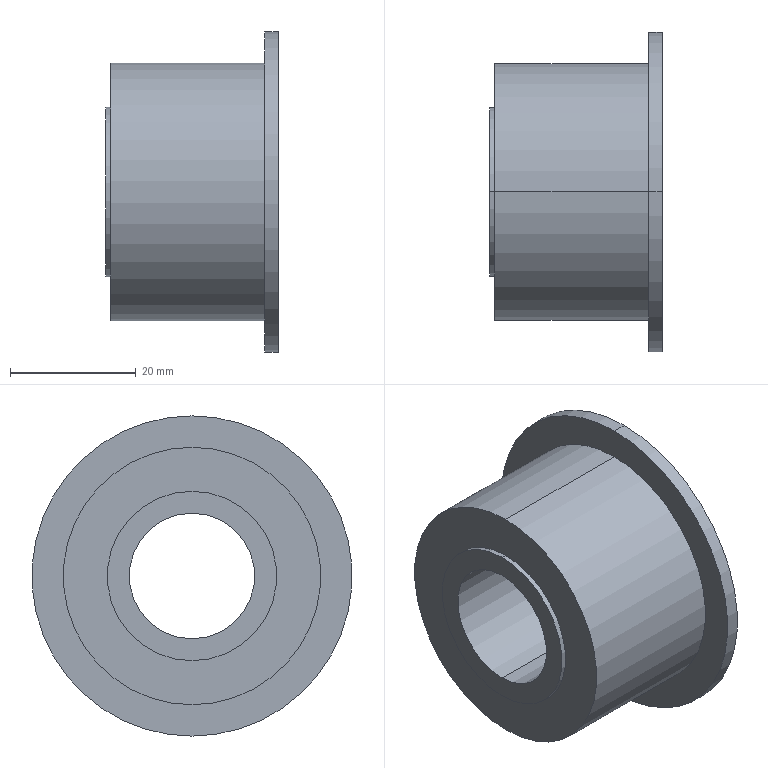Part | SolidWorks | features Revolution 1 | 1 solid | 18 faces | box 27.5 x 51 x 51 mm | volume 16998 mm3 | cylinder 12 | plane 6 | commonest cylinder face diameters 27 x4 20 x2 37 x2 41 x2 51 x2
STEP:
#1=CARTESIAN_POINT('',(27.5,0.,-18.5));
#2=VERTEX_POINT('',#1);
#3=CARTESIAN_POINT('',(27.5,0.,18.5));
#4=VERTEX_POINT('',#3);
#5=CARTESIAN_POINT('',(27.5,0.,0.));
#6=DIRECTION('',(-1.,0.,0.));
#7=DIRECTION('',(0.,0.,1.));
#8=AXIS2_PLACEMENT_3D('',#5,#6,#7);
#9=CIRCLE('',#8,18.5);
#10=EDGE_CURVE('',#2,#4,#9,.T.);
#11=ORIENTED_EDGE('',*,*,#10,.F.);
#12=CARTESIAN_POINT('',(4.3,0.,-18.5));
#13=VERTEX_POINT('',#12);
#14=CARTESIAN_POINT('',(0.,0.,-18.5));
#15=DIRECTION('',(-1.,0.,0.));
#16=VECTOR('',#15,1000.);
#17=LINE('',#14,#16);
#18=EDGE_CURVE('',#2,#13,#17,.T.);
#19=ORIENTED_EDGE('',*,*,#18,.T.);
#20=CARTESIAN_POINT('',(4.3,0.,18.5));
#21=VERTEX_POINT('',#20);
#22=CARTESIAN_POINT('',(4.3,0.,0.));
#23=DIRECTION('',(-1.,0.,0.));
#24=DIRECTION('',(0.,0.,1.));
#25=AXIS2_PLACEMENT_3D('',#22,#23,#24);
#26=CIRCLE('',#25,18.5);
#27=EDGE_CURVE('',#13,#21,#26,.T.);
#28=ORIENTED_EDGE('',*,*,#27,.T.);
#29=CARTESIAN_POINT('',(0.,0.,18.5));
#30=DIRECTION('',(-1.,0.,0.));
#31=VECTOR('',#30,1000.);
#32=LINE('',#29,#31);
#33=EDGE_CURVE('',#4,#21,#32,.T.);
#34=ORIENTED_EDGE('',*,*,#33,.F.);
#35=EDGE_LOOP('',(#11,#19,#28,#34));
#36=FACE_OUTER_BOUND('',#35,.T.);
#37=CARTESIAN_POINT('',(0.,0.,0.));
#38=DIRECTION('',(-1.,0.,0.));
#39=DIRECTION('',(0.,0.,1.));
#40=AXIS2_PLACEMENT_3D('',#37,#38,#39);
#41=CYLINDRICAL_SURFACE('',#40,18.5);
#42=ADVANCED_FACE('',(#36),#41,.F.);
#43=CARTESIAN_POINT('',(27.5,0.,13.5));
#44=VERTEX_POINT('',#43);
#45=CARTESIAN_POINT('',(27.5,0.,-13.5));
#46=VERTEX_POINT('',#45);
#47=CARTESIAN_POINT('',(27.5,0.,0.));
#48=DIRECTION('',(-1.,0.,0.));
#49=DIRECTION('',(0.,0.,1.));
#50=AXIS2_PLACEMENT_3D('',#47,#48,#49);
#51=CIRCLE('',#50,13.5);
#52=EDGE_CURVE('',#44,#46,#51,.T.);
#53=ORIENTED_EDGE('',*,*,#52,.T.);
#54=CARTESIAN_POINT('',(4.3,0.,-13.5));
#55=VERTEX_POINT('',#54);
#56=CARTESIAN_POINT('',(0.,0.,-13.5));
#57=DIRECTION('',(-1.,0.,0.));
#58=VECTOR('',#57,1000.);
#59=LINE('',#56,#58);
#60=EDGE_CURVE('',#46,#55,#59,.T.);
#61=ORIENTED_EDGE('',*,*,#60,.T.);
#62=CARTESIAN_POINT('',(4.3,0.,13.5));
#63=VERTEX_POINT('',#62);
#64=CARTESIAN_POINT('',(4.3,0.,0.));
#65=DIRECTION('',(-1.,0.,0.));
#66=DIRECTION('',(0.,0.,1.));
#67=AXIS2_PLACEMENT_3D('',#64,#65,#66);
#68=CIRCLE('',#67,13.5);
#69=EDGE_CURVE('',#63,#55,#68,.T.);
#70=ORIENTED_EDGE('',*,*,#69,.F.);
#71=CARTESIAN_POINT('',(0.,0.,13.5));
#72=DIRECTION('',(-1.,0.,0.));
#73=VECTOR('',#72,1000.);
#74=LINE('',#71,#73);
#75=EDGE_CURVE('',#44,#63,#74,.T.);
#76=ORIENTED_EDGE('',*,*,#75,.F.);
#77=EDGE_LOOP('',(#53,#61,#70,#76));
#78=FACE_OUTER_BOUND('',#77,.T.);
#79=CARTESIAN_POINT('',(0.,0.,0.));
#80=DIRECTION('',(-1.,0.,0.));
#81=DIRECTION('',(0.,0.,1.));
#82=AXIS2_PLACEMENT_3D('',#79,#80,#81);
#83=CYLINDRICAL_SURFACE('',#82,13.5);
#84=ADVANCED_FACE('',(#78),#83,.T.);
#85=CARTESIAN_POINT('',(27.5,0.,-10.));
#86=VERTEX_POINT('',#85);
#87=CARTESIAN_POINT('',(27.5,0.,10.));
#88=VERTEX_POINT('',#87);
#89=CARTESIAN_POINT('',(27.5,0.,0.));
#90=DIRECTION('',(-1.,0.,0.));
#91=DIRECTION('',(0.,0.,1.));
#92=AXIS2_PLACEMENT_3D('',#89,#90,#91);
#93=CIRCLE('',#92,10.);
#94=EDGE_CURVE('',#86,#88,#93,.T.);
#95=ORIENTED_EDGE('',*,*,#94,.F.);
#96=CARTESIAN_POINT('',(0.,0.,-10.));
#97=VERTEX_POINT('',#96);
#98=CARTESIAN_POINT('',(0.,0.,-10.));
#99=DIRECTION('',(-1.,0.,0.));
#100=VECTOR('',#99,1000.);
#101=LINE('',#98,#100);
#102=EDGE_CURVE('',#86,#97,#101,.T.);
#103=ORIENTED_EDGE('',*,*,#102,.T.);
#104=CARTESIAN_POINT('',(0.,0.,10.));
#105=VERTEX_POINT('',#104);
#106=CARTESIAN_POINT('',(0.,0.,0.));
#107=DIRECTION('',(-1.,0.,0.));
#108=DIRECTION('',(0.,0.,1.));
#109=AXIS2_PLACEMENT_3D('',#106,#107,#108);
#110=CIRCLE('',#109,10.);
#111=EDGE_CURVE('',#97,#105,#110,.T.);
#112=ORIENTED_EDGE('',*,*,#111,.T.);
#113=CARTESIAN_POINT('',(0.,0.,10.));
#114=DIRECTION('',(-1.,0.,0.));
#115=VECTOR('',#114,1000.);
#116=LINE('',#113,#115);
#117=EDGE_CURVE('',#88,#105,#116,.T.);
#118=ORIENTED_EDGE('',*,*,#117,.F.);
#119=EDGE_LOOP('',(#95,#103,#112,#118));
#120=FACE_OUTER_BOUND('',#119,.T.);
#121=CARTESIAN_POINT('',(0.,0.,0.));
#122=DIRECTION('',(-1.,0.,0.));
#123=DIRECTION('',(0.,0.,1.));
#124=AXIS2_PLACEMENT_3D('',#121,#122,#123);
#125=CYLINDRICAL_SURFACE('',#124,10.);
#126=ADVANCED_FACE('',(#120),#125,.F.);
#127=CARTESIAN_POINT('',(0.8,0.,13.5));
#128=VERTEX_POINT('',#127);
#129=CARTESIAN_POINT('',(0.8,0.,-13.5));
#130=VERTEX_POINT('',#129);
#131=CARTESIAN_POINT('',(0.8,0.,0.));
#132=DIRECTION('',(-1.,0.,0.));
#133=DIRECTION('',(0.,0.,1.));
#134=AXIS2_PLACEMENT_3D('',#131,#132,#133);
#135=CIRCLE('',#134,13.5);
#136=EDGE_CURVE('',#128,#130,#135,.T.);
#137=ORIENTED_EDGE('',*,*,#136,.T.);
#138=CARTESIAN_POINT('',(0.,0.,-13.5));
#139=VERTEX_POINT('',#138);
#140=CARTESIAN_POINT('',(0.,0.,-13.5));
#141=DIRECTION('',(-1.,0.,0.));
#142=VECTOR('',#141,1000.);
#143=LINE('',#140,#142);
#144=EDGE_CURVE('',#130,#139,#143,.T.);
#145=ORIENTED_EDGE('',*,*,#144,.T.);
#146=CARTESIAN_POINT('',(0.,0.,13.5));
#147=VERTEX_POINT('',#146);
#148=CARTESIAN_POINT('',(0.,0.,0.));
#149=DIRECTION('',(-1.,0.,0.));
#150=DIRECTION('',(0.,0.,1.));
#151=AXIS2_PLACEMENT_3D('',#148,#149,#150);
#152=CIRCLE('',#151,13.5);
#153=EDGE_CURVE('',#147,#139,#152,.T.);
#154=ORIENTED_EDGE('',*,*,#153,.F.);
#155=CARTESIAN_POINT('',(0.,0.,13.5));
#156=DIRECTION('',(-1.,0.,0.));
#157=VECTOR('',#156,1000.);
#158=LINE('',#155,#157);
#159=EDGE_CURVE('',#128,#147,#158,.T.);
#160=ORIENTED_EDGE('',*,*,#159,.F.);
#161=EDGE_LOOP('',(#137,#145,#154,#160));
#162=FACE_OUTER_BOUND('',#161,.T.);
#163=CARTESIAN_POINT('',(0.,0.,0.));
#164=DIRECTION('',(-1.,0.,0.));
#165=DIRECTION('',(0.,0.,1.));
#166=AXIS2_PLACEMENT_3D('',#163,#164,#165);
#167=CYLINDRICAL_SURFACE('',#166,13.5);
#168=ADVANCED_FACE('',(#162),#167,.T.);
#169=CARTESIAN_POINT('',(25.3,0.,20.5));
#170=VERTEX_POINT('',#169);
#171=CARTESIAN_POINT('',(25.3,0.,-20.5));
#172=VERTEX_POINT('',#171);
#173=CARTESIAN_POINT('',(25.3,0.,0.));
#174=DIRECTION('',(-1.,0.,0.));
#175=DIRECTION('',(0.,0.,1.));
#176=AXIS2_PLACEMENT_3D('',#173,#174,#175);
#177=CIRCLE('',#176,20.5);
#178=EDGE_CURVE('',#170,#172,#177,.T.);
#179=ORIENTED_EDGE('',*,*,#178,.T.);
#180=CARTESIAN_POINT('',(0.8,0.,-20.5));
#181=VERTEX_POINT('',#180);
#182=CARTESIAN_POINT('',(0.,0.,-20.5));
#183=DIRECTION('',(-1.,0.,0.));
#184=VECTOR('',#183,1000.);
#185=LINE('',#182,#184);
#186=EDGE_CURVE('',#172,#181,#185,.T.);
#187=ORIENTED_EDGE('',*,*,#186,.T.);
#188=CARTESIAN_POINT('',(0.8,0.,20.5));
#189=VERTEX_POINT('',#188);
#190=CARTESIAN_POINT('',(0.8,0.,0.));
#191=DIRECTION('',(-1.,0.,0.));
#192=DIRECTION('',(0.,0.,1.));
#193=AXIS2_PLACEMENT_3D('',#190,#191,#192);
#194=CIRCLE('',#193,20.5);
#195=EDGE_CURVE('',#189,#181,#194,.T.);
#196=ORIENTED_EDGE('',*,*,#195,.F.);
#197=CARTESIAN_POINT('',(0.,0.,20.5));
#198=DIRECTION('',(-1.,0.,0.));
#199=VECTOR('',#198,1000.);
#200=LINE('',#197,#199);
#201=EDGE_CURVE('',#170,#189,#200,.T.);
#202=ORIENTED_EDGE('',*,*,#201,.F.);
#203=EDGE_LOOP('',(#179,#187,#196,#202));
#204=FACE_OUTER_BOUND('',#203,.T.);
#205=CARTESIAN_POINT('',(0.,0.,0.));
#206=DIRECTION('',(-1.,0.,0.));
#207=DIRECTION('',(0.,0.,1.));
#208=AXIS2_PLACEMENT_3D('',#205,#206,#207);
#209=CYLINDRICAL_SURFACE('',#208,20.5);
#210=ADVANCED_FACE('',(#204),#209,.T.);
#211=CARTESIAN_POINT('',(27.5,0.,25.5));
#212=VERTEX_POINT('',#211);
#213=CARTESIAN_POINT('',(27.5,0.,-25.5));
#214=VERTEX_POINT('',#213);
#215=CARTESIAN_POINT('',(27.5,0.,0.));
#216=DIRECTION('',(-1.,0.,0.));
#217=DIRECTION('',(0.,0.,1.));
#218=AXIS2_PLACEMENT_3D('',#215,#216,#217);
#219=CIRCLE('',#218,25.5);
#220=EDGE_CURVE('',#212,#214,#219,.T.);
#221=ORIENTED_EDGE('',*,*,#220,.T.);
#222=CARTESIAN_POINT('',(25.3,0.,-25.5));
#223=VERTEX_POINT('',#222);
#224=CARTESIAN_POINT('',(0.,0.,-25.5));
#225=DIRECTION('',(-1.,0.,0.));
#226=VECTOR('',#225,1000.);
#227=LINE('',#224,#226);
#228=EDGE_CURVE('',#214,#223,#227,.T.);
#229=ORIENTED_EDGE('',*,*,#228,.T.);
#230=CARTESIAN_POINT('',(25.3,0.,25.5));
#231=VERTEX_POINT('',#230);
#232=CARTESIAN_POINT('',(25.3,0.,0.));
#233=DIRECTION('',(-1.,0.,0.));
#234=DIRECTION('',(0.,0.,1.));
#235=AXIS2_PLACEMENT_3D('',#232,#233,#234);
#236=CIRCLE('',#235,25.5);
#237=EDGE_CURVE('',#231,#223,#236,.T.);
#238=ORIENTED_EDGE('',*,*,#237,.F.);
#239=CARTESIAN_POINT('',(0.,0.,25.5));
#240=DIRECTION('',(-1.,0.,0.));
#241=VECTOR('',#240,1000.);
#242=LINE('',#239,#241);
#243=EDGE_CURVE('',#212,#231,#242,.T.);
#244=ORIENTED_EDGE('',*,*,#243,.F.);
#245=EDGE_LOOP('',(#221,#229,#238,#244));
#246=FACE_OUTER_BOUND('',#245,.T.);
#247=CARTESIAN_POINT('',(0.,0.,0.));
#248=DIRECTION('',(-1.,0.,0.));
#249=DIRECTION('',(0.,0.,1.));
#250=AXIS2_PLACEMENT_3D('',#247,#248,#249);
#251=CYLINDRICAL_SURFACE('',#250,25.5);
#252=ADVANCED_FACE('',(#246),#251,.T.);
#253=ORIENTED_EDGE('',*,*,#228,.F.);
#254=CARTESIAN_POINT('',(27.5,0.,0.));
#255=DIRECTION('',(-1.,0.,0.));
#256=DIRECTION('',(0.,0.,1.));
#257=AXIS2_PLACEMENT_3D('',#254,#255,#256);
#258=CIRCLE('',#257,25.5);
#259=EDGE_CURVE('',#214,#212,#258,.T.);
#260=ORIENTED_EDGE('',*,*,#259,.T.);
#261=ORIENTED_EDGE('',*,*,#243,.T.);
#262=CARTESIAN_POINT('',(25.3,0.,0.));
#263=DIRECTION('',(-1.,0.,0.));
#264=DIRECTION('',(0.,0.,1.));
#265=AXIS2_PLACEMENT_3D('',#262,#263,#264);
#266=CIRCLE('',#265,25.5);
#267=EDGE_CURVE('',#223,#231,#266,.T.);
#268=ORIENTED_EDGE('',*,*,#267,.F.);
#269=EDGE_LOOP('',(#253,#260,#261,#268));
#270=FACE_OUTER_BOUND('',#269,.T.);
#271=CARTESIAN_POINT('',(0.,0.,0.));
#272=DIRECTION('',(-1.,0.,0.));
#273=DIRECTION('',(0.,0.,1.));
#274=AXIS2_PLACEMENT_3D('',#271,#272,#273);
#275=CYLINDRICAL_SURFACE('',#274,25.5);
#276=ADVANCED_FACE('',(#270),#275,.T.);
#277=ORIENTED_EDGE('',*,*,#178,.F.);
#278=CARTESIAN_POINT('',(25.3,0.,0.));
#279=DIRECTION('',(-1.,0.,0.));
#280=DIRECTION('',(0.,0.,1.));
#281=AXIS2_PLACEMENT_3D('',#278,#279,#280);
#282=CIRCLE('',#281,20.5);
#283=EDGE_CURVE('',#172,#170,#282,.T.);
#284=ORIENTED_EDGE('',*,*,#283,.F.);
#285=EDGE_LOOP('',(#277,#284));
#286=FACE_BOUND('',#285,.T.);
#287=ORIENTED_EDGE('',*,*,#237,.T.);
#288=ORIENTED_EDGE('',*,*,#267,.T.);
#289=EDGE_LOOP('',(#287,#288));
#290=FACE_OUTER_BOUND('',#289,.T.);
#291=CARTESIAN_POINT('',(25.3,25.5,0.));
#292=DIRECTION('',(1.,0.,0.));
#293=DIRECTION('',(0.,0.,-1.));
#294=AXIS2_PLACEMENT_3D('',#291,#292,#293);
#295=PLANE('',#294);
#296=ADVANCED_FACE('',(#286,#290),#295,.F.);
#297=ORIENTED_EDGE('',*,*,#186,.F.);
#298=ORIENTED_EDGE('',*,*,#283,.T.);
#299=ORIENTED_EDGE('',*,*,#201,.T.);
#300=CARTESIAN_POINT('',(0.8,0.,0.));
#301=DIRECTION('',(-1.,0.,0.));
#302=DIRECTION('',(0.,0.,1.));
#303=AXIS2_PLACEMENT_3D('',#300,#301,#302);
#304=CIRCLE('',#303,20.5);
#305=EDGE_CURVE('',#181,#189,#304,.T.);
#306=ORIENTED_EDGE('',*,*,#305,.F.);
#307=EDGE_LOOP('',(#297,#298,#299,#306));
#308=FACE_OUTER_BOUND('',#307,.T.);
#309=CARTESIAN_POINT('',(0.,0.,0.));
#310=DIRECTION('',(-1.,0.,0.));
#311=DIRECTION('',(0.,0.,1.));
#312=AXIS2_PLACEMENT_3D('',#309,#310,#311);
#313=CYLINDRICAL_SURFACE('',#312,20.5);
#314=ADVANCED_FACE('',(#308),#313,.T.);
#315=ORIENTED_EDGE('',*,*,#136,.F.);
#316=CARTESIAN_POINT('',(0.8,0.,0.));
#317=DIRECTION('',(-1.,0.,0.));
#318=DIRECTION('',(0.,0.,1.));
#319=AXIS2_PLACEMENT_3D('',#316,#317,#318);
#320=CIRCLE('',#319,13.5);
#321=EDGE_CURVE('',#130,#128,#320,.T.);
#322=ORIENTED_EDGE('',*,*,#321,.F.);
#323=EDGE_LOOP('',(#315,#322));
#324=FACE_BOUND('',#323,.T.);
#325=ORIENTED_EDGE('',*,*,#195,.T.);
#326=ORIENTED_EDGE('',*,*,#305,.T.);
#327=EDGE_LOOP('',(#325,#326));
#328=FACE_OUTER_BOUND('',#327,.T.);
#329=CARTESIAN_POINT('',(0.8,20.5,0.));
#330=DIRECTION('',(1.,0.,0.));
#331=DIRECTION('',(0.,0.,-1.));
#332=AXIS2_PLACEMENT_3D('',#329,#330,#331);
#333=PLANE('',#332);
#334=ADVANCED_FACE('',(#324,#328),#333,.F.);
#335=ORIENTED_EDGE('',*,*,#144,.F.);
#336=ORIENTED_EDGE('',*,*,#321,.T.);
#337=ORIENTED_EDGE('',*,*,#159,.T.);
#338=CARTESIAN_POINT('',(0.,0.,0.));
#339=DIRECTION('',(-1.,0.,0.));
#340=DIRECTION('',(0.,0.,1.));
#341=AXIS2_PLACEMENT_3D('',#338,#339,#340);
#342=CIRCLE('',#341,13.5);
#343=EDGE_CURVE('',#139,#147,#342,.T.);
#344=ORIENTED_EDGE('',*,*,#343,.F.);
#345=EDGE_LOOP('',(#335,#336,#337,#344));
#346=FACE_OUTER_BOUND('',#345,.T.);
#347=CARTESIAN_POINT('',(0.,0.,0.));
#348=DIRECTION('',(-1.,0.,0.));
#349=DIRECTION('',(0.,0.,1.));
#350=AXIS2_PLACEMENT_3D('',#347,#348,#349);
#351=CYLINDRICAL_SURFACE('',#350,13.5);
#352=ADVANCED_FACE('',(#346),#351,.T.);
#353=CARTESIAN_POINT('',(0.,0.,0.));
#354=DIRECTION('',(-1.,0.,0.));
#355=DIRECTION('',(0.,0.,1.));
#356=AXIS2_PLACEMENT_3D('',#353,#354,#355);
#357=CIRCLE('',#356,10.);
#358=EDGE_CURVE('',#105,#97,#357,.T.);
#359=ORIENTED_EDGE('',*,*,#358,.F.);
#360=ORIENTED_EDGE('',*,*,#111,.F.);
#361=EDGE_LOOP('',(#359,#360));
#362=FACE_BOUND('',#361,.T.);
#363=ORIENTED_EDGE('',*,*,#153,.T.);
#364=ORIENTED_EDGE('',*,*,#343,.T.);
#365=EDGE_LOOP('',(#363,#364));
#366=FACE_OUTER_BOUND('',#365,.T.);
#367=CARTESIAN_POINT('',(0.,13.5,0.));
#368=DIRECTION('',(1.,0.,0.));
#369=DIRECTION('',(0.,0.,-1.));
#370=AXIS2_PLACEMENT_3D('',#367,#368,#369);
#371=PLANE('',#370);
#372=ADVANCED_FACE('',(#362,#366),#371,.F.);
#373=ORIENTED_EDGE('',*,*,#102,.F.);
#374=CARTESIAN_POINT('',(27.5,0.,0.));
#375=DIRECTION('',(-1.,0.,0.));
#376=DIRECTION('',(0.,0.,1.));
#377=AXIS2_PLACEMENT_3D('',#374,#375,#376);
#378=CIRCLE('',#377,10.);
#379=EDGE_CURVE('',#88,#86,#378,.T.);
#380=ORIENTED_EDGE('',*,*,#379,.F.);
#381=ORIENTED_EDGE('',*,*,#117,.T.);
#382=ORIENTED_EDGE('',*,*,#358,.T.);
#383=EDGE_LOOP('',(#373,#380,#381,#382));
#384=FACE_OUTER_BOUND('',#383,.T.);
#385=CARTESIAN_POINT('',(0.,0.,0.));
#386=DIRECTION('',(-1.,0.,0.));
#387=DIRECTION('',(0.,0.,1.));
#388=AXIS2_PLACEMENT_3D('',#385,#386,#387);
#389=CYLINDRICAL_SURFACE('',#388,10.);
#390=ADVANCED_FACE('',(#384),#389,.F.);
#391=ORIENTED_EDGE('',*,*,#52,.F.);
#392=CARTESIAN_POINT('',(27.5,0.,0.));
#393=DIRECTION('',(-1.,0.,0.));
#394=DIRECTION('',(0.,0.,1.));
#395=AXIS2_PLACEMENT_3D('',#392,#393,#394);
#396=CIRCLE('',#395,13.5);
#397=EDGE_CURVE('',#46,#44,#396,.T.);
#398=ORIENTED_EDGE('',*,*,#397,.F.);
#399=EDGE_LOOP('',(#391,#398));
#400=FACE_OUTER_BOUND('',#399,.T.);
#401=ORIENTED_EDGE('',*,*,#379,.T.);
#402=ORIENTED_EDGE('',*,*,#94,.T.);
#403=EDGE_LOOP('',(#401,#402));
#404=FACE_BOUND('',#403,.T.);
#405=CARTESIAN_POINT('',(27.5,10.,0.));
#406=DIRECTION('',(-1.,0.,0.));
#407=DIRECTION('',(0.,0.,1.));
#408=AXIS2_PLACEMENT_3D('',#405,#406,#407);
#409=PLANE('',#408);
#410=ADVANCED_FACE('',(#400,#404),#409,.F.);
#411=ORIENTED_EDGE('',*,*,#60,.F.);
#412=ORIENTED_EDGE('',*,*,#397,.T.);
#413=ORIENTED_EDGE('',*,*,#75,.T.);
#414=CARTESIAN_POINT('',(4.3,0.,0.));
#415=DIRECTION('',(-1.,0.,0.));
#416=DIRECTION('',(0.,0.,1.));
#417=AXIS2_PLACEMENT_3D('',#414,#415,#416);
#418=CIRCLE('',#417,13.5);
#419=EDGE_CURVE('',#55,#63,#418,.T.);
#420=ORIENTED_EDGE('',*,*,#419,.F.);
#421=EDGE_LOOP('',(#411,#412,#413,#420));
#422=FACE_OUTER_BOUND('',#421,.T.);
#423=CARTESIAN_POINT('',(0.,0.,0.));
#424=DIRECTION('',(-1.,0.,0.));
#425=DIRECTION('',(0.,0.,1.));
#426=AXIS2_PLACEMENT_3D('',#423,#424,#425);
#427=CYLINDRICAL_SURFACE('',#426,13.5);
#428=ADVANCED_FACE('',(#422),#427,.T.);
#429=CARTESIAN_POINT('',(4.3,0.,0.));
#430=DIRECTION('',(-1.,0.,0.));
#431=DIRECTION('',(0.,0.,1.));
#432=AXIS2_PLACEMENT_3D('',#429,#430,#431);
#433=CIRCLE('',#432,18.5);
#434=EDGE_CURVE('',#21,#13,#433,.T.);
#435=ORIENTED_EDGE('',*,*,#434,.F.);
#436=ORIENTED_EDGE('',*,*,#27,.F.);
#437=EDGE_LOOP('',(#435,#436));
#438=FACE_OUTER_BOUND('',#437,.T.);
#439=ORIENTED_EDGE('',*,*,#69,.T.);
#440=ORIENTED_EDGE('',*,*,#419,.T.);
#441=EDGE_LOOP('',(#439,#440));
#442=FACE_BOUND('',#441,.T.);
#443=CARTESIAN_POINT('',(4.3,13.5,0.));
#444=DIRECTION('',(-1.,0.,0.));
#445=DIRECTION('',(0.,0.,1.));
#446=AXIS2_PLACEMENT_3D('',#443,#444,#445);
#447=PLANE('',#446);
#448=ADVANCED_FACE('',(#438,#442),#447,.F.);
#449=ORIENTED_EDGE('',*,*,#18,.F.);
#450=CARTESIAN_POINT('',(27.5,0.,0.));
#451=DIRECTION('',(-1.,0.,0.));
#452=DIRECTION('',(0.,0.,1.));
#453=AXIS2_PLACEMENT_3D('',#450,#451,#452);
#454=CIRCLE('',#453,18.5);
#455=EDGE_CURVE('',#4,#2,#454,.T.);
#456=ORIENTED_EDGE('',*,*,#455,.F.);
#457=ORIENTED_EDGE('',*,*,#33,.T.);
#458=ORIENTED_EDGE('',*,*,#434,.T.);
#459=EDGE_LOOP('',(#449,#456,#457,#458));
#460=FACE_OUTER_BOUND('',#459,.T.);
#461=CARTESIAN_POINT('',(0.,0.,0.));
#462=DIRECTION('',(-1.,0.,0.));
#463=DIRECTION('',(0.,0.,1.));
#464=AXIS2_PLACEMENT_3D('',#461,#462,#463);
#465=CYLINDRICAL_SURFACE('',#464,18.5);
#466=ADVANCED_FACE('',(#460),#465,.F.);
#467=ORIENTED_EDGE('',*,*,#220,.F.);
#468=ORIENTED_EDGE('',*,*,#259,.F.);
#469=EDGE_LOOP('',(#467,#468));
#470=FACE_OUTER_BOUND('',#469,.T.);
#471=ORIENTED_EDGE('',*,*,#455,.T.);
#472=ORIENTED_EDGE('',*,*,#10,.T.);
#473=EDGE_LOOP('',(#471,#472));
#474=FACE_BOUND('',#473,.T.);
#475=CARTESIAN_POINT('',(27.5,18.5,0.));
#476=DIRECTION('',(-1.,0.,0.));
#477=DIRECTION('',(0.,0.,1.));
#478=AXIS2_PLACEMENT_3D('',#475,#476,#477);
#479=PLANE('',#478);
#480=ADVANCED_FACE('',(#470,#474),#479,.F.);
#481=CLOSED_SHELL('',(#42,#84,#126,#168,#210,#252,#276,#296,#314,#334,#352,#372,#390,#410,#428,#448,#466,#480));
#482=MANIFOLD_SOLID_BREP('',#481);
#483=CARTESIAN_POINT('',(0.,0.,0.));
#484=DIRECTION('',(0.,0.,1.));
#485=DIRECTION('',(1.,0.,0.));
#486=AXIS2_PLACEMENT_3D('',#483,#484,#485);
#487=(LENGTH_UNIT()NAMED_UNIT(*)SI_UNIT(.MILLI.,.METRE.));
#488=UNCERTAINTY_MEASURE_WITH_UNIT(LENGTH_MEASURE(0.00001),#487,'','');
#489=(NAMED_UNIT(*)PLANE_ANGLE_UNIT()SI_UNIT($,.RADIAN.));
#490=(NAMED_UNIT(*)SI_UNIT($,.STERADIAN.)SOLID_ANGLE_UNIT());
#491=(GEOMETRIC_REPRESENTATION_CONTEXT(3)GLOBAL_UNCERTAINTY_ASSIGNED_CONTEXT((#488))GLOBAL_UNIT_ASSIGNED_CONTEXT((#487,#489,#490))REPRESENTATION_CONTEXT('',''));
#492=ADVANCED_BREP_SHAPE_REPRESENTATION('',(#482,#486),#491);